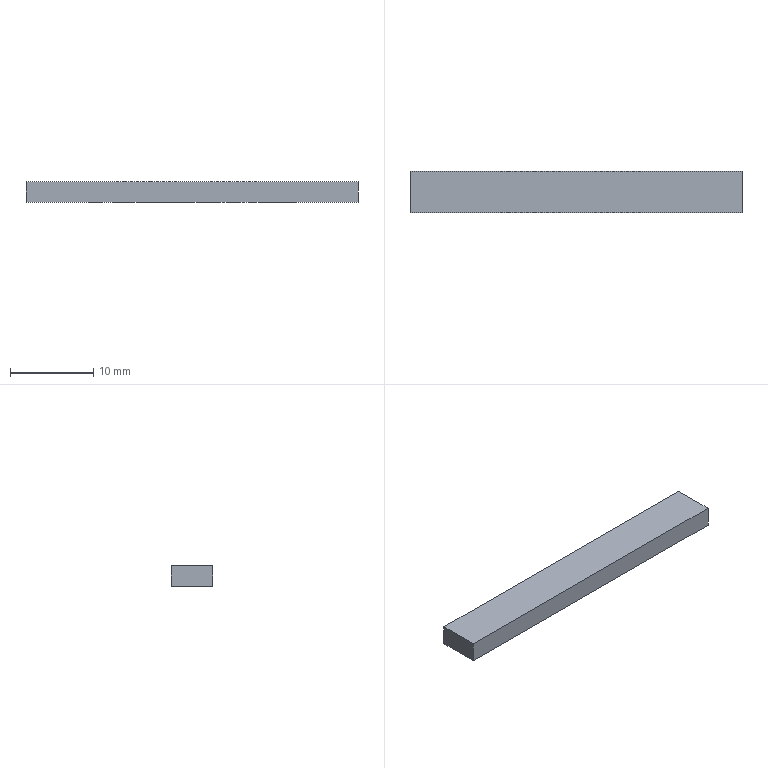Part | STEP file | lll_id998_x_t | 1 solid | 72 faces | box 40 x 5 x 2.5 mm | volume 497.143 mm3 | plane 51 | other 21